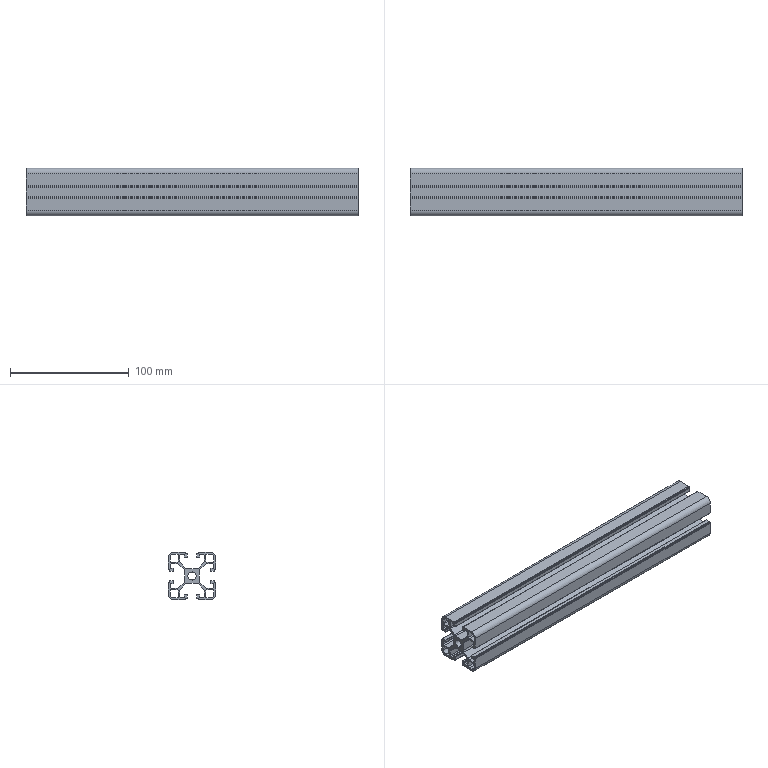Part | STEP file | MK-8-4040C-L-00 profile 4040C standard 280mm | 1 solid | 188 faces | box 280 x 40 x 40 mm | volume 133910 mm3 | cylinder 94 | plane 94 | commonest cylinder face diameters 0.6 x30 2 x28 4 x16 0.4 x8 6 x4 9 x4